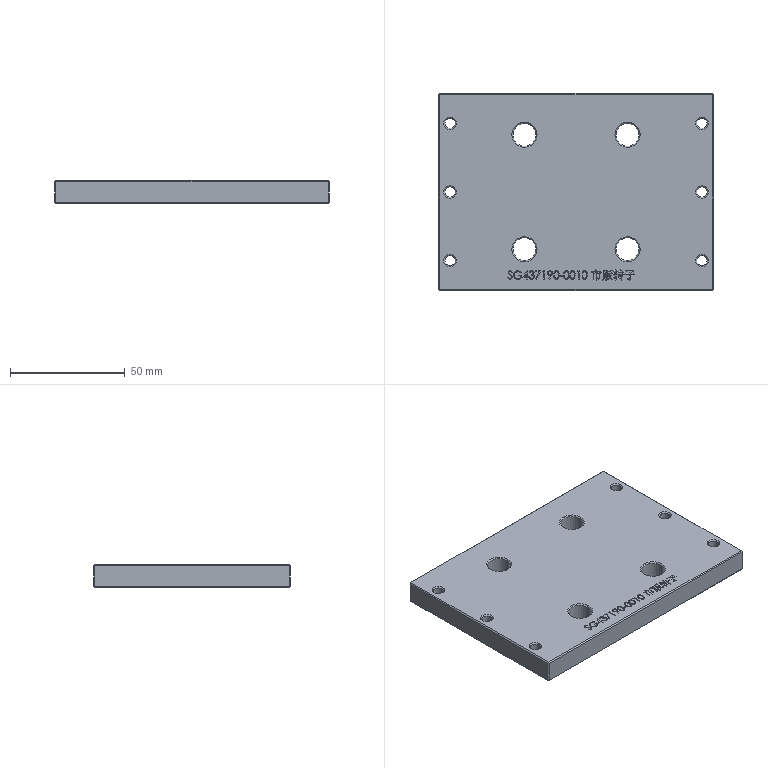Part | STEP file | Base plate-market rotor circlip | 1 solid | 438 faces | box 120 x 86 x 10 mm | volume 97902 mm3 | plane 234 | spline 132 | cone 40 | cylinder 32 | commonest cylinder face diameters 4.5 x12 8 x12 10 x8